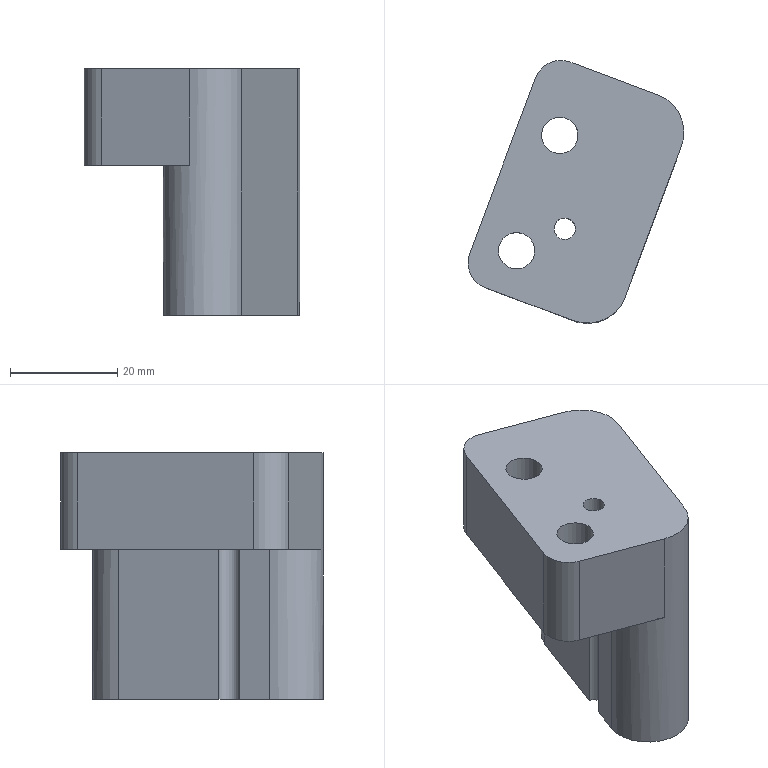Part | NX | features solid 2 | 1 solid | 24 faces | box 40.273 x 49.07 x 46 mm | volume 37890 mm3 | plane 11 | cylinder 11 | cone 2 | commonest cylinder face diameters 5.199 x2 6.8 x2 10 x2 11 x2 15 x2 4.001 x1
STEP:
#1=CARTESIAN_POINT('',(340.887,34.527,53.));
#2=VERTEX_POINT('',#1);
#3=CARTESIAN_POINT('',(336.736,38.135,53.));
#4=DIRECTION('',(0.000000102,-0.000000038,1.));
#5=DIRECTION('',(0.7547,-0.6561,-0.000000102));
#6=AXIS2_PLACEMENT_3D('',#3,#4,#5);
#7=CIRCLE('',#6,5.5);
#8=EDGE_CURVE('',#2,#2,#7,.T.);
#9=ORIENTED_EDGE('',*,*,#8,.T.);
#10=EDGE_LOOP('',(#9));
#11=FACE_BOUND('',#10,.T.);
#12=CARTESIAN_POINT('',(342.943,34.747,53.));
#13=VERTEX_POINT('',#12);
#14=CARTESIAN_POINT('',(345.044,40.367,53.));
#15=VERTEX_POINT('',#14);
#16=CARTESIAN_POINT('',(344.256,38.26,53.));
#17=DIRECTION('',(0.3502,0.9367,0.));
#18=VECTOR('',#17,1000.);
#19=LINE('',#16,#18);
#20=EDGE_CURVE('',#13,#15,#19,.T.);
#21=ORIENTED_EDGE('',*,*,#20,.F.);
#22=CARTESIAN_POINT('',(347.341,25.096,53.));
#23=VERTEX_POINT('',#22);
#24=CARTESIAN_POINT('',(349.968,32.121,53.));
#25=DIRECTION('',(0.,0.,-1.));
#26=DIRECTION('',(-1.,0.,0.));
#27=AXIS2_PLACEMENT_3D('',#24,#25,#26);
#28=CIRCLE('',#27,7.5);
#29=EDGE_CURVE('',#23,#13,#28,.T.);
#30=ORIENTED_EDGE('',*,*,#29,.F.);
#31=CARTESIAN_POINT('',(330.95,31.224,53.));
#32=VERTEX_POINT('',#31);
#33=CARTESIAN_POINT('',(328.608,32.1,53.));
#34=DIRECTION('',(0.9367,-0.3502,-0.000000109));
#35=VECTOR('',#34,1000.);
#36=LINE('',#33,#35);
#37=EDGE_CURVE('',#32,#23,#36,.T.);
#38=ORIENTED_EDGE('',*,*,#37,.F.);
#39=CARTESIAN_POINT('',(328.017,37.659,53.));
#40=VERTEX_POINT('',#39);
#41=CARTESIAN_POINT('',(332.701,35.908,53.));
#42=DIRECTION('',(0.000000102,-0.000000038,1.));
#43=DIRECTION('',(-1.,0.,0.000000102));
#44=AXIS2_PLACEMENT_3D('',#41,#42,#43);
#45=CIRCLE('',#44,5.);
#46=EDGE_CURVE('',#40,#32,#45,.T.);
#47=ORIENTED_EDGE('',*,*,#46,.F.);
#48=CARTESIAN_POINT('',(340.274,70.442,53.));
#49=VERTEX_POINT('',#48);
#50=CARTESIAN_POINT('',(362.919,131.008,53.));
#51=DIRECTION('',(-0.3502,-0.9367,0.));
#52=VECTOR('',#51,1000.);
#53=LINE('',#50,#52);
#54=EDGE_CURVE('',#49,#40,#53,.T.);
#55=ORIENTED_EDGE('',*,*,#54,.F.);
#56=CARTESIAN_POINT('',(346.709,73.375,53.));
#57=VERTEX_POINT('',#56);
#58=CARTESIAN_POINT('',(344.958,68.691,53.));
#59=DIRECTION('',(0.000000102,-0.000000038,1.));
#60=DIRECTION('',(-1.,0.,0.000000102));
#61=AXIS2_PLACEMENT_3D('',#58,#59,#60);
#62=CIRCLE('',#61,5.);
#63=EDGE_CURVE('',#57,#49,#62,.T.);
#64=ORIENTED_EDGE('',*,*,#63,.F.);
#65=CARTESIAN_POINT('',(363.101,67.246,53.));
#66=VERTEX_POINT('',#65);
#67=CARTESIAN_POINT('',(344.367,74.25,53.));
#68=DIRECTION('',(0.9367,-0.3502,-0.000000109));
#69=VECTOR('',#68,1000.);
#70=LINE('',#67,#69);
#71=EDGE_CURVE('',#57,#66,#70,.T.);
#72=ORIENTED_EDGE('',*,*,#71,.T.);
#73=CARTESIAN_POINT('',(353.449,62.847,53.));
#74=VERTEX_POINT('',#73);
#75=CARTESIAN_POINT('',(360.474,60.221,53.));
#76=DIRECTION('',(0.,0.,1.));
#77=DIRECTION('',(-1.,0.,0.));
#78=AXIS2_PLACEMENT_3D('',#75,#76,#77);
#79=CIRCLE('',#78,7.5);
#80=EDGE_CURVE('',#66,#74,#79,.T.);
#81=ORIENTED_EDGE('',*,*,#80,.T.);
#82=CARTESIAN_POINT('',(346.445,44.114,53.));
#83=VERTEX_POINT('',#82);
#84=CARTESIAN_POINT('',(344.256,38.26,53.));
#85=DIRECTION('',(0.3502,0.9367,0.));
#86=VECTOR('',#85,1000.);
#87=LINE('',#84,#86);
#88=EDGE_CURVE('',#83,#74,#87,.T.);
#89=ORIENTED_EDGE('',*,*,#88,.F.);
#90=CARTESIAN_POINT('',(345.744,42.241,53.));
#91=DIRECTION('',(-0.000000102,0.000000038,-1.));
#92=DIRECTION('',(-1.,0.,0.000000102));
#93=AXIS2_PLACEMENT_3D('',#90,#91,#92);
#94=CIRCLE('',#93,2.001);
#95=EDGE_CURVE('',#15,#83,#94,.T.);
#96=ORIENTED_EDGE('',*,*,#95,.F.);
#97=EDGE_LOOP('',(#21,#30,#38,#47,#55,#64,#72,#81,#89,#96));
#98=FACE_BOUND('',#97,.T.);
#99=CARTESIAN_POINT('',(350.291,59.679,53.));
#100=VERTEX_POINT('',#99);
#101=CARTESIAN_POINT('',(344.791,59.679,53.));
#102=DIRECTION('',(-0.000000102,0.000000038,-1.));
#103=DIRECTION('',(1.,0.,-0.000000102));
#104=AXIS2_PLACEMENT_3D('',#101,#102,#103);
#105=CIRCLE('',#104,5.5);
#106=EDGE_CURVE('',#100,#100,#105,.T.);
#107=ORIENTED_EDGE('',*,*,#106,.F.);
#108=EDGE_LOOP('',(#107));
#109=FACE_BOUND('',#108,.T.);
#110=CARTESIAN_POINT('',(365.26,130.133,53.));
#111=DIRECTION('',(-0.000000102,0.000000038,-1.));
#112=DIRECTION('',(1.,0.,-0.000000102));
#113=AXIS2_PLACEMENT_3D('',#110,#111,#112);
#114=PLANE('',#113);
#115=ADVANCED_FACE('',(#11,#98,#109),#114,.T.);
#116=CARTESIAN_POINT('',(340.136,38.135,71.));
#117=VERTEX_POINT('',#116);
#118=CARTESIAN_POINT('',(336.736,38.135,71.));
#119=DIRECTION('',(-0.000000102,0.000000038,-1.));
#120=DIRECTION('',(1.,0.,-0.000000102));
#121=AXIS2_PLACEMENT_3D('',#118,#119,#120);
#122=CIRCLE('',#121,3.4);
#123=EDGE_CURVE('',#117,#117,#122,.T.);
#124=ORIENTED_EDGE('',*,*,#123,.T.);
#125=EDGE_LOOP('',(#124));
#126=FACE_BOUND('',#125,.T.);
#127=CARTESIAN_POINT('',(330.95,31.224,71.));
#128=VERTEX_POINT('',#127);
#129=CARTESIAN_POINT('',(347.341,25.096,71.));
#130=VERTEX_POINT('',#129);
#131=CARTESIAN_POINT('',(328.608,32.1,71.));
#132=DIRECTION('',(0.9367,-0.3502,-0.000000109));
#133=VECTOR('',#132,1000.);
#134=LINE('',#131,#133);
#135=EDGE_CURVE('',#128,#130,#134,.T.);
#136=ORIENTED_EDGE('',*,*,#135,.T.);
#137=CARTESIAN_POINT('',(356.993,29.494,71.));
#138=VERTEX_POINT('',#137);
#139=CARTESIAN_POINT('',(349.968,32.121,71.));
#140=DIRECTION('',(0.,0.,1.));
#141=DIRECTION('',(1.,0.,0.));
#142=AXIS2_PLACEMENT_3D('',#139,#140,#141);
#143=CIRCLE('',#142,7.5);
#144=EDGE_CURVE('',#130,#138,#143,.T.);
#145=ORIENTED_EDGE('',*,*,#144,.T.);
#146=CARTESIAN_POINT('',(367.499,57.594,71.));
#147=VERTEX_POINT('',#146);
#148=CARTESIAN_POINT('',(358.306,33.007,71.));
#149=DIRECTION('',(0.3502,0.9367,0.));
#150=VECTOR('',#149,1000.);
#151=LINE('',#148,#150);
#152=EDGE_CURVE('',#138,#147,#151,.T.);
#153=ORIENTED_EDGE('',*,*,#152,.T.);
#154=CARTESIAN_POINT('',(363.101,67.246,71.));
#155=VERTEX_POINT('',#154);
#156=CARTESIAN_POINT('',(360.474,60.221,71.));
#157=DIRECTION('',(0.,0.,1.));
#158=DIRECTION('',(1.,0.,0.));
#159=AXIS2_PLACEMENT_3D('',#156,#157,#158);
#160=CIRCLE('',#159,7.5);
#161=EDGE_CURVE('',#147,#155,#160,.T.);
#162=ORIENTED_EDGE('',*,*,#161,.T.);
#163=CARTESIAN_POINT('',(346.709,73.375,71.));
#164=VERTEX_POINT('',#163);
#165=CARTESIAN_POINT('',(344.367,74.25,71.));
#166=DIRECTION('',(0.9367,-0.3502,-0.000000109));
#167=VECTOR('',#166,1000.);
#168=LINE('',#165,#167);
#169=EDGE_CURVE('',#164,#155,#168,.T.);
#170=ORIENTED_EDGE('',*,*,#169,.F.);
#171=CARTESIAN_POINT('',(340.274,70.442,71.));
#172=VERTEX_POINT('',#171);
#173=CARTESIAN_POINT('',(344.958,68.691,71.));
#174=DIRECTION('',(-0.000000102,0.000000038,-1.));
#175=DIRECTION('',(1.,0.,-0.000000102));
#176=AXIS2_PLACEMENT_3D('',#173,#174,#175);
#177=CIRCLE('',#176,5.);
#178=EDGE_CURVE('',#172,#164,#177,.T.);
#179=ORIENTED_EDGE('',*,*,#178,.F.);
#180=CARTESIAN_POINT('',(328.017,37.659,71.));
#181=VERTEX_POINT('',#180);
#182=CARTESIAN_POINT('',(362.919,131.008,71.));
#183=DIRECTION('',(0.3502,0.9367,0.));
#184=VECTOR('',#183,1000.);
#185=LINE('',#182,#184);
#186=EDGE_CURVE('',#181,#172,#185,.T.);
#187=ORIENTED_EDGE('',*,*,#186,.F.);
#188=CARTESIAN_POINT('',(332.701,35.908,71.));
#189=DIRECTION('',(-0.000000102,0.000000038,-1.));
#190=DIRECTION('',(1.,0.,-0.000000102));
#191=AXIS2_PLACEMENT_3D('',#188,#189,#190);
#192=CIRCLE('',#191,5.);
#193=EDGE_CURVE('',#128,#181,#192,.T.);
#194=ORIENTED_EDGE('',*,*,#193,.F.);
#195=EDGE_LOOP('',(#136,#145,#153,#162,#170,#179,#187,#194));
#196=FACE_BOUND('',#195,.T.);
#197=CARTESIAN_POINT('',(347.745,42.241,71.));
#198=VERTEX_POINT('',#197);
#199=CARTESIAN_POINT('',(345.744,42.241,71.));
#200=DIRECTION('',(-0.000000102,0.000000038,-1.));
#201=DIRECTION('',(1.,0.,-0.000000102));
#202=AXIS2_PLACEMENT_3D('',#199,#200,#201);
#203=CIRCLE('',#202,2.001);
#204=EDGE_CURVE('',#198,#198,#203,.T.);
#205=ORIENTED_EDGE('',*,*,#204,.T.);
#206=EDGE_LOOP('',(#205));
#207=FACE_BOUND('',#206,.T.);
#208=CARTESIAN_POINT('',(348.191,59.679,71.));
#209=VERTEX_POINT('',#208);
#210=CARTESIAN_POINT('',(344.791,59.679,71.));
#211=DIRECTION('',(0.000000102,-0.000000038,1.));
#212=DIRECTION('',(1.,0.,-0.000000102));
#213=AXIS2_PLACEMENT_3D('',#210,#211,#212);
#214=CIRCLE('',#213,3.4);
#215=EDGE_CURVE('',#209,#209,#214,.T.);
#216=ORIENTED_EDGE('',*,*,#215,.F.);
#217=EDGE_LOOP('',(#216));
#218=FACE_BOUND('',#217,.T.);
#219=CARTESIAN_POINT('',(365.26,130.133,71.));
#220=DIRECTION('',(0.000000102,-0.000000038,1.));
#221=DIRECTION('',(-1.,0.,0.000000102));
#222=AXIS2_PLACEMENT_3D('',#219,#220,#221);
#223=PLANE('',#222);
#224=ADVANCED_FACE('',(#126,#196,#207,#218),#223,.T.);
#225=CARTESIAN_POINT('',(346.445,44.114,25.));
#226=VERTEX_POINT('',#225);
#227=CARTESIAN_POINT('',(346.445,44.114,15.));
#228=DIRECTION('',(0.000000103,-0.000000037,1.));
#229=VECTOR('',#228,1000.);
#230=LINE('',#227,#229);
#231=EDGE_CURVE('',#226,#83,#230,.T.);
#232=ORIENTED_EDGE('',*,*,#231,.T.);
#233=ORIENTED_EDGE('',*,*,#88,.T.);
#234=CARTESIAN_POINT('',(353.449,62.847,25.));
#235=VERTEX_POINT('',#234);
#236=CARTESIAN_POINT('',(353.449,62.847,65.));
#237=DIRECTION('',(-0.000000103,0.000000037,-1.));
#238=VECTOR('',#237,1000.);
#239=LINE('',#236,#238);
#240=EDGE_CURVE('',#74,#235,#239,.T.);
#241=ORIENTED_EDGE('',*,*,#240,.T.);
#242=CARTESIAN_POINT('',(344.256,38.26,25.));
#243=DIRECTION('',(0.3502,0.9367,-0.000000001));
#244=VECTOR('',#243,1000.);
#245=LINE('',#242,#244);
#246=EDGE_CURVE('',#226,#235,#245,.T.);
#247=ORIENTED_EDGE('',*,*,#246,.F.);
#248=EDGE_LOOP('',(#232,#233,#241,#247));
#249=FACE_BOUND('',#248,.T.);
#250=CARTESIAN_POINT('',(344.256,38.26,65.));
#251=DIRECTION('',(0.9367,-0.3502,-0.000000109));
#252=DIRECTION('',(0.3502,0.9367,0.));
#253=AXIS2_PLACEMENT_3D('',#250,#251,#252);
#254=PLANE('',#253);
#255=ADVANCED_FACE('',(#249),#254,.F.);
#256=CARTESIAN_POINT('',(345.044,40.367,25.));
#257=VERTEX_POINT('',#256);
#258=CARTESIAN_POINT('',(345.044,40.367,15.));
#259=DIRECTION('',(-0.000000103,0.000000037,-1.));
#260=VECTOR('',#259,1000.);
#261=LINE('',#258,#260);
#262=EDGE_CURVE('',#15,#257,#261,.T.);
#263=ORIENTED_EDGE('',*,*,#262,.T.);
#264=CARTESIAN_POINT('',(342.943,34.747,25.));
#265=VERTEX_POINT('',#264);
#266=CARTESIAN_POINT('',(344.256,38.26,25.));
#267=DIRECTION('',(0.3502,0.9367,-0.000000001));
#268=VECTOR('',#267,1000.);
#269=LINE('',#266,#268);
#270=EDGE_CURVE('',#265,#257,#269,.T.);
#271=ORIENTED_EDGE('',*,*,#270,.F.);
#272=CARTESIAN_POINT('',(342.943,34.747,65.));
#273=DIRECTION('',(-0.000000103,0.000000037,-1.));
#274=VECTOR('',#273,1000.);
#275=LINE('',#272,#274);
#276=EDGE_CURVE('',#13,#265,#275,.T.);
#277=ORIENTED_EDGE('',*,*,#276,.F.);
#278=ORIENTED_EDGE('',*,*,#20,.T.);
#279=EDGE_LOOP('',(#263,#271,#277,#278));
#280=FACE_BOUND('',#279,.T.);
#281=CARTESIAN_POINT('',(344.256,38.26,65.));
#282=DIRECTION('',(0.9367,-0.3502,-0.000000109));
#283=DIRECTION('',(0.3502,0.9367,0.));
#284=AXIS2_PLACEMENT_3D('',#281,#282,#283);
#285=PLANE('',#284);
#286=ADVANCED_FACE('',(#280),#285,.F.);
#287=CARTESIAN_POINT('',(352.568,32.121,25.));
#288=VERTEX_POINT('',#287);
#289=CARTESIAN_POINT('',(349.968,32.121,25.));
#290=DIRECTION('',(0.000000103,-0.000000037,1.));
#291=DIRECTION('',(1.,0.,-0.000000103));
#292=AXIS2_PLACEMENT_3D('',#289,#290,#291);
#293=CIRCLE('',#292,2.599);
#294=EDGE_CURVE('',#288,#288,#293,.T.);
#295=ORIENTED_EDGE('',*,*,#294,.T.);
#296=EDGE_LOOP('',(#295));
#297=FACE_BOUND('',#296,.T.);
#298=CARTESIAN_POINT('',(363.074,60.221,25.));
#299=VERTEX_POINT('',#298);
#300=CARTESIAN_POINT('',(360.474,60.221,25.));
#301=DIRECTION('',(0.000000103,-0.000000037,1.));
#302=DIRECTION('',(1.,0.,-0.000000103));
#303=AXIS2_PLACEMENT_3D('',#300,#301,#302);
#304=CIRCLE('',#303,2.599);
#305=EDGE_CURVE('',#299,#299,#304,.T.);
#306=ORIENTED_EDGE('',*,*,#305,.T.);
#307=EDGE_LOOP('',(#306));
#308=FACE_BOUND('',#307,.T.);
#309=CARTESIAN_POINT('',(345.744,42.241,25.));
#310=DIRECTION('',(0.000000103,-0.000000037,1.));
#311=DIRECTION('',(1.,0.,-0.000000103));
#312=AXIS2_PLACEMENT_3D('',#309,#310,#311);
#313=CIRCLE('',#312,2.001);
#314=EDGE_CURVE('',#257,#226,#313,.T.);
#315=ORIENTED_EDGE('',*,*,#314,.T.);
#316=ORIENTED_EDGE('',*,*,#246,.T.);
#317=CARTESIAN_POINT('',(367.499,57.594,25.));
#318=VERTEX_POINT('',#317);
#319=CARTESIAN_POINT('',(360.474,60.221,25.));
#320=DIRECTION('',(0.000000103,-0.000000037,1.));
#321=DIRECTION('',(1.,0.,-0.000000103));
#322=AXIS2_PLACEMENT_3D('',#319,#320,#321);
#323=CIRCLE('',#322,7.5);
#324=EDGE_CURVE('',#318,#235,#323,.T.);
#325=ORIENTED_EDGE('',*,*,#324,.F.);
#326=CARTESIAN_POINT('',(356.993,29.494,25.));
#327=VERTEX_POINT('',#326);
#328=CARTESIAN_POINT('',(358.306,33.007,25.));
#329=DIRECTION('',(0.3502,0.9367,-0.000000001));
#330=VECTOR('',#329,1000.);
#331=LINE('',#328,#330);
#332=EDGE_CURVE('',#327,#318,#331,.T.);
#333=ORIENTED_EDGE('',*,*,#332,.F.);
#334=CARTESIAN_POINT('',(349.968,32.121,25.));
#335=DIRECTION('',(0.000000103,-0.000000037,1.));
#336=DIRECTION('',(1.,0.,-0.000000103));
#337=AXIS2_PLACEMENT_3D('',#334,#335,#336);
#338=CIRCLE('',#337,7.5);
#339=EDGE_CURVE('',#265,#327,#338,.T.);
#340=ORIENTED_EDGE('',*,*,#339,.F.);
#341=ORIENTED_EDGE('',*,*,#270,.T.);
#342=EDGE_LOOP('',(#315,#316,#325,#333,#340,#341));
#343=FACE_BOUND('',#342,.T.);
#344=CARTESIAN_POINT('',(351.281,35.633,25.));
#345=DIRECTION('',(0.000000103,-0.000000037,1.));
#346=DIRECTION('',(-0.04361,-0.999,-0.000000033));
#347=AXIS2_PLACEMENT_3D('',#344,#345,#346);
#348=PLANE('',#347);
#349=ADVANCED_FACE('',(#297,#308,#343),#348,.F.);
#350=ORIENTED_EDGE('',*,*,#29,.T.);
#351=ORIENTED_EDGE('',*,*,#276,.T.);
#352=ORIENTED_EDGE('',*,*,#339,.T.);
#353=CARTESIAN_POINT('',(356.993,29.494,65.));
#354=DIRECTION('',(-0.000000103,0.000000037,-1.));
#355=VECTOR('',#354,1000.);
#356=LINE('',#353,#355);
#357=EDGE_CURVE('',#138,#327,#356,.T.);
#358=ORIENTED_EDGE('',*,*,#357,.F.);
#359=ORIENTED_EDGE('',*,*,#144,.F.);
#360=CARTESIAN_POINT('',(347.341,25.096,65.));
#361=DIRECTION('',(0.000000103,-0.000000037,1.));
#362=VECTOR('',#361,1000.);
#363=LINE('',#360,#362);
#364=EDGE_CURVE('',#23,#130,#363,.T.);
#365=ORIENTED_EDGE('',*,*,#364,.F.);
#366=EDGE_LOOP('',(#350,#351,#352,#358,#359,#365));
#367=FACE_BOUND('',#366,.T.);
#368=CARTESIAN_POINT('',(349.968,32.121,65.));
#369=DIRECTION('',(-0.000000103,0.000000037,-1.));
#370=DIRECTION('',(1.,0.,-0.000000103));
#371=AXIS2_PLACEMENT_3D('',#368,#369,#370);
#372=CYLINDRICAL_SURFACE('',#371,7.5);
#373=ADVANCED_FACE('',(#367),#372,.T.);
#374=CARTESIAN_POINT('',(367.499,57.594,65.));
#375=DIRECTION('',(-0.000000103,0.000000037,-1.));
#376=VECTOR('',#375,1000.);
#377=LINE('',#374,#376);
#378=EDGE_CURVE('',#147,#318,#377,.T.);
#379=ORIENTED_EDGE('',*,*,#378,.T.);
#380=ORIENTED_EDGE('',*,*,#324,.T.);
#381=ORIENTED_EDGE('',*,*,#240,.F.);
#382=ORIENTED_EDGE('',*,*,#80,.F.);
#383=CARTESIAN_POINT('',(363.101,67.246,65.));
#384=DIRECTION('',(-0.000000103,0.000000037,-1.));
#385=VECTOR('',#384,1000.);
#386=LINE('',#383,#385);
#387=EDGE_CURVE('',#155,#66,#386,.T.);
#388=ORIENTED_EDGE('',*,*,#387,.F.);
#389=ORIENTED_EDGE('',*,*,#161,.F.);
#390=EDGE_LOOP('',(#379,#380,#381,#382,#388,#389));
#391=FACE_BOUND('',#390,.T.);
#392=CARTESIAN_POINT('',(360.474,60.221,65.));
#393=DIRECTION('',(-0.000000103,0.000000037,-1.));
#394=DIRECTION('',(1.,0.,-0.000000103));
#395=AXIS2_PLACEMENT_3D('',#392,#393,#394);
#396=CYLINDRICAL_SURFACE('',#395,7.5);
#397=ADVANCED_FACE('',(#391),#396,.T.);
#398=ORIENTED_EDGE('',*,*,#357,.T.);
#399=ORIENTED_EDGE('',*,*,#332,.T.);
#400=ORIENTED_EDGE('',*,*,#378,.F.);
#401=ORIENTED_EDGE('',*,*,#152,.F.);
#402=EDGE_LOOP('',(#398,#399,#400,#401));
#403=FACE_BOUND('',#402,.T.);
#404=CARTESIAN_POINT('',(358.306,33.007,65.));
#405=DIRECTION('',(0.9367,-0.3502,-0.000000109));
#406=DIRECTION('',(0.3502,0.9367,0.));
#407=AXIS2_PLACEMENT_3D('',#404,#405,#406);
#408=PLANE('',#407);
#409=ADVANCED_FACE('',(#403),#408,.T.);
#410=ORIENTED_EDGE('',*,*,#169,.T.);
#411=ORIENTED_EDGE('',*,*,#387,.T.);
#412=ORIENTED_EDGE('',*,*,#71,.F.);
#413=CARTESIAN_POINT('',(346.709,73.375,65.));
#414=DIRECTION('',(-0.000000103,0.000000037,-1.));
#415=VECTOR('',#414,1000.);
#416=LINE('',#413,#415);
#417=EDGE_CURVE('',#164,#57,#416,.T.);
#418=ORIENTED_EDGE('',*,*,#417,.F.);
#419=EDGE_LOOP('',(#410,#411,#412,#418));
#420=FACE_BOUND('',#419,.T.);
#421=CARTESIAN_POINT('',(344.367,74.25,65.));
#422=DIRECTION('',(0.3502,0.9367,-0.000000001));
#423=DIRECTION('',(-0.9367,0.3502,0.));
#424=AXIS2_PLACEMENT_3D('',#421,#422,#423);
#425=PLANE('',#424);
#426=ADVANCED_FACE('',(#420),#425,.T.);
#427=ORIENTED_EDGE('',*,*,#37,.T.);
#428=ORIENTED_EDGE('',*,*,#364,.T.);
#429=ORIENTED_EDGE('',*,*,#135,.F.);
#430=CARTESIAN_POINT('',(330.95,31.224,65.));
#431=DIRECTION('',(0.000000103,-0.000000037,1.));
#432=VECTOR('',#431,1000.);
#433=LINE('',#430,#432);
#434=EDGE_CURVE('',#32,#128,#433,.T.);
#435=ORIENTED_EDGE('',*,*,#434,.F.);
#436=EDGE_LOOP('',(#427,#428,#429,#435));
#437=FACE_BOUND('',#436,.T.);
#438=CARTESIAN_POINT('',(328.608,32.1,65.));
#439=DIRECTION('',(-0.3502,-0.9367,0.000000001));
#440=DIRECTION('',(0.9367,-0.3502,0.));
#441=AXIS2_PLACEMENT_3D('',#438,#439,#440);
#442=PLANE('',#441);
#443=ADVANCED_FACE('',(#437),#442,.T.);
#444=ORIENTED_EDGE('',*,*,#186,.T.);
#445=CARTESIAN_POINT('',(340.274,70.442,53.));
#446=DIRECTION('',(0.000000103,-0.000000037,1.));
#447=VECTOR('',#446,1000.);
#448=LINE('',#445,#447);
#449=EDGE_CURVE('',#49,#172,#448,.T.);
#450=ORIENTED_EDGE('',*,*,#449,.F.);
#451=ORIENTED_EDGE('',*,*,#54,.T.);
#452=CARTESIAN_POINT('',(328.017,37.659,53.));
#453=DIRECTION('',(-0.000000103,0.000000037,-1.));
#454=VECTOR('',#453,1000.);
#455=LINE('',#452,#454);
#456=EDGE_CURVE('',#181,#40,#455,.T.);
#457=ORIENTED_EDGE('',*,*,#456,.F.);
#458=EDGE_LOOP('',(#444,#450,#451,#457));
#459=FACE_BOUND('',#458,.T.);
#460=CARTESIAN_POINT('',(328.893,40.,53.));
#461=DIRECTION('',(-0.9367,0.3502,0.000000109));
#462=DIRECTION('',(-0.3502,-0.9367,0.));
#463=AXIS2_PLACEMENT_3D('',#460,#461,#462);
#464=PLANE('',#463);
#465=ADVANCED_FACE('',(#459),#464,.T.);
#466=ORIENTED_EDGE('',*,*,#46,.T.);
#467=ORIENTED_EDGE('',*,*,#434,.T.);
#468=ORIENTED_EDGE('',*,*,#193,.T.);
#469=ORIENTED_EDGE('',*,*,#456,.T.);
#470=EDGE_LOOP('',(#466,#467,#468,#469));
#471=FACE_BOUND('',#470,.T.);
#472=CARTESIAN_POINT('',(332.701,35.908,65.));
#473=DIRECTION('',(0.000000103,-0.000000037,1.));
#474=DIRECTION('',(-1.,0.,0.000000103));
#475=AXIS2_PLACEMENT_3D('',#472,#473,#474);
#476=CYLINDRICAL_SURFACE('',#475,5.);
#477=ADVANCED_FACE('',(#471),#476,.T.);
#478=ORIENTED_EDGE('',*,*,#178,.T.);
#479=ORIENTED_EDGE('',*,*,#417,.T.);
#480=ORIENTED_EDGE('',*,*,#63,.T.);
#481=ORIENTED_EDGE('',*,*,#449,.T.);
#482=EDGE_LOOP('',(#478,#479,#480,#481));
#483=FACE_BOUND('',#482,.T.);
#484=CARTESIAN_POINT('',(344.958,68.691,65.));
#485=DIRECTION('',(-0.000000103,0.000000037,-1.));
#486=DIRECTION('',(1.,0.,-0.000000103));
#487=AXIS2_PLACEMENT_3D('',#484,#485,#486);
#488=CYLINDRICAL_SURFACE('',#487,5.);
#489=ADVANCED_FACE('',(#483),#488,.T.);
#490=ORIENTED_EDGE('',*,*,#204,.F.);
#491=EDGE_LOOP('',(#490));
#492=FACE_BOUND('',#491,.T.);
#493=ORIENTED_EDGE('',*,*,#314,.F.);
#494=ORIENTED_EDGE('',*,*,#262,.F.);
#495=ORIENTED_EDGE('',*,*,#95,.T.);
#496=ORIENTED_EDGE('',*,*,#231,.F.);
#497=EDGE_LOOP('',(#493,#494,#495,#496));
#498=FACE_BOUND('',#497,.T.);
#499=CARTESIAN_POINT('',(345.744,42.241,15.));
#500=DIRECTION('',(-0.000000103,0.000000037,-1.));
#501=DIRECTION('',(1.,0.,-0.000000103));
#502=AXIS2_PLACEMENT_3D('',#499,#500,#501);
#503=CYLINDRICAL_SURFACE('',#502,2.001);
#504=ADVANCED_FACE('',(#492,#498),#503,.F.);
#505=CARTESIAN_POINT('',(348.191,59.679,62.));
#506=VERTEX_POINT('',#505);
#507=CARTESIAN_POINT('',(344.791,59.679,62.));
#508=DIRECTION('',(-0.000000102,0.000000038,-1.));
#509=DIRECTION('',(1.,0.,-0.000000102));
#510=AXIS2_PLACEMENT_3D('',#507,#508,#509);
#511=CIRCLE('',#510,3.4);
#512=EDGE_CURVE('',#506,#506,#511,.T.);
#513=ORIENTED_EDGE('',*,*,#512,.T.);
#514=EDGE_LOOP('',(#513));
#515=FACE_BOUND('',#514,.T.);
#516=ORIENTED_EDGE('',*,*,#215,.T.);
#517=EDGE_LOOP('',(#516));
#518=FACE_BOUND('',#517,.T.);
#519=CARTESIAN_POINT('',(344.791,59.679,53.));
#520=DIRECTION('',(0.000000102,-0.000000038,1.));
#521=DIRECTION('',(-1.,0.,0.000000102));
#522=AXIS2_PLACEMENT_3D('',#519,#520,#521);
#523=CYLINDRICAL_SURFACE('',#522,3.4);
#524=ADVANCED_FACE('',(#515,#518),#523,.F.);
#525=ORIENTED_EDGE('',*,*,#512,.F.);
#526=EDGE_LOOP('',(#525));
#527=FACE_BOUND('',#526,.T.);
#528=CARTESIAN_POINT('',(350.291,59.679,62.));
#529=VERTEX_POINT('',#528);
#530=CARTESIAN_POINT('',(344.791,59.679,62.));
#531=DIRECTION('',(-0.000000102,0.000000038,-1.));
#532=DIRECTION('',(1.,0.,-0.000000102));
#533=AXIS2_PLACEMENT_3D('',#530,#531,#532);
#534=CIRCLE('',#533,5.5);
#535=EDGE_CURVE('',#529,#529,#534,.T.);
#536=ORIENTED_EDGE('',*,*,#535,.T.);
#537=EDGE_LOOP('',(#536));
#538=FACE_BOUND('',#537,.T.);
#539=CARTESIAN_POINT('',(344.791,59.679,62.));
#540=DIRECTION('',(0.000000102,-0.000000038,1.));
#541=DIRECTION('',(-1.,0.,0.000000102));
#542=AXIS2_PLACEMENT_3D('',#539,#540,#541);
#543=PLANE('',#542);
#544=ADVANCED_FACE('',(#527,#538),#543,.F.);
#545=ORIENTED_EDGE('',*,*,#535,.F.);
#546=EDGE_LOOP('',(#545));
#547=FACE_BOUND('',#546,.T.);
#548=ORIENTED_EDGE('',*,*,#106,.T.);
#549=EDGE_LOOP('',(#548));
#550=FACE_BOUND('',#549,.T.);
#551=CARTESIAN_POINT('',(344.791,59.679,53.));
#552=DIRECTION('',(0.000000102,-0.000000038,1.));
#553=DIRECTION('',(-1.,0.,0.000000102));
#554=AXIS2_PLACEMENT_3D('',#551,#552,#553);
#555=CYLINDRICAL_SURFACE('',#554,5.5);
#556=ADVANCED_FACE('',(#547,#550),#555,.F.);
#557=CARTESIAN_POINT('',(340.136,38.135,62.));
#558=VERTEX_POINT('',#557);
#559=CARTESIAN_POINT('',(336.736,38.135,62.));
#560=DIRECTION('',(0.000000102,-0.000000038,1.));
#561=DIRECTION('',(1.,0.,-0.000000102));
#562=AXIS2_PLACEMENT_3D('',#559,#560,#561);
#563=CIRCLE('',#562,3.4);
#564=EDGE_CURVE('',#558,#558,#563,.T.);
#565=ORIENTED_EDGE('',*,*,#564,.F.);
#566=EDGE_LOOP('',(#565));
#567=FACE_BOUND('',#566,.T.);
#568=ORIENTED_EDGE('',*,*,#123,.F.);
#569=EDGE_LOOP('',(#568));
#570=FACE_BOUND('',#569,.T.);
#571=CARTESIAN_POINT('',(336.736,38.135,53.));
#572=DIRECTION('',(0.000000102,-0.000000038,1.));
#573=DIRECTION('',(-0.7547,0.6561,0.000000102));
#574=AXIS2_PLACEMENT_3D('',#571,#572,#573);
#575=CYLINDRICAL_SURFACE('',#574,3.4);
#576=ADVANCED_FACE('',(#567,#570),#575,.F.);
#577=ORIENTED_EDGE('',*,*,#564,.T.);
#578=EDGE_LOOP('',(#577));
#579=FACE_BOUND('',#578,.T.);
#580=CARTESIAN_POINT('',(340.887,34.527,62.));
#581=VERTEX_POINT('',#580);
#582=CARTESIAN_POINT('',(336.736,38.135,62.));
#583=DIRECTION('',(0.000000102,-0.000000038,1.));
#584=DIRECTION('',(0.7547,-0.6561,-0.000000102));
#585=AXIS2_PLACEMENT_3D('',#582,#583,#584);
#586=CIRCLE('',#585,5.5);
#587=EDGE_CURVE('',#581,#581,#586,.T.);
#588=ORIENTED_EDGE('',*,*,#587,.F.);
#589=EDGE_LOOP('',(#588));
#590=FACE_BOUND('',#589,.T.);
#591=CARTESIAN_POINT('',(336.736,38.135,62.));
#592=DIRECTION('',(0.000000102,-0.000000038,1.));
#593=DIRECTION('',(-0.7547,0.6561,0.000000102));
#594=AXIS2_PLACEMENT_3D('',#591,#592,#593);
#595=PLANE('',#594);
#596=ADVANCED_FACE('',(#579,#590),#595,.F.);
#597=ORIENTED_EDGE('',*,*,#587,.T.);
#598=EDGE_LOOP('',(#597));
#599=FACE_BOUND('',#598,.T.);
#600=ORIENTED_EDGE('',*,*,#8,.F.);
#601=EDGE_LOOP('',(#600));
#602=FACE_BOUND('',#601,.T.);
#603=CARTESIAN_POINT('',(336.736,38.135,53.));
#604=DIRECTION('',(0.000000102,-0.000000038,1.));
#605=DIRECTION('',(-0.7547,0.6561,0.000000102));
#606=AXIS2_PLACEMENT_3D('',#603,#604,#605);
#607=CYLINDRICAL_SURFACE('',#606,5.5);
#608=ADVANCED_FACE('',(#599,#602),#607,.F.);
#609=CARTESIAN_POINT('',(363.074,60.221,37.401));
#610=VERTEX_POINT('',#609);
#611=CARTESIAN_POINT('',(360.474,60.221,37.401));
#612=DIRECTION('',(0.000000103,-0.000000037,1.));
#613=DIRECTION('',(1.,0.,-0.000000103));
#614=AXIS2_PLACEMENT_3D('',#611,#612,#613);
#615=CIRCLE('',#614,2.599);
#616=EDGE_CURVE('',#610,#610,#615,.T.);
#617=ORIENTED_EDGE('',*,*,#616,.T.);
#618=EDGE_LOOP('',(#617));
#619=FACE_BOUND('',#618,.T.);
#620=ORIENTED_EDGE('',*,*,#305,.F.);
#621=EDGE_LOOP('',(#620));
#622=FACE_BOUND('',#621,.T.);
#623=CARTESIAN_POINT('',(360.474,60.221,25.));
#624=DIRECTION('',(0.000000103,-0.000000037,1.));
#625=DIRECTION('',(-1.,0.,0.000000103));
#626=AXIS2_PLACEMENT_3D('',#623,#624,#625);
#627=CYLINDRICAL_SURFACE('',#626,2.599);
#628=ADVANCED_FACE('',(#619,#622),#627,.F.);
#629=CARTESIAN_POINT('',(360.474,60.221,40.));
#630=VERTEX_POINT('',#629);
#631=VERTEX_LOOP('',#630);
#632=FACE_BOUND('',#631,.T.);
#633=ORIENTED_EDGE('',*,*,#616,.F.);
#634=EDGE_LOOP('',(#633));
#635=FACE_BOUND('',#634,.T.);
#636=CARTESIAN_POINT('',(360.474,60.221,37.401));
#637=DIRECTION('',(-0.000000103,0.000000037,-1.));
#638=DIRECTION('',(1.,0.,-0.000000103));
#639=AXIS2_PLACEMENT_3D('',#636,#637,#638);
#640=CONICAL_SURFACE('',#639,2.599,0.7854);
#641=ADVANCED_FACE('',(#632,#635),#640,.F.);
#642=CARTESIAN_POINT('',(352.568,32.121,37.401));
#643=VERTEX_POINT('',#642);
#644=CARTESIAN_POINT('',(349.968,32.121,37.401));
#645=DIRECTION('',(0.000000103,-0.000000037,1.));
#646=DIRECTION('',(1.,0.,-0.000000103));
#647=AXIS2_PLACEMENT_3D('',#644,#645,#646);
#648=CIRCLE('',#647,2.599);
#649=EDGE_CURVE('',#643,#643,#648,.T.);
#650=ORIENTED_EDGE('',*,*,#649,.T.);
#651=EDGE_LOOP('',(#650));
#652=FACE_BOUND('',#651,.T.);
#653=ORIENTED_EDGE('',*,*,#294,.F.);
#654=EDGE_LOOP('',(#653));
#655=FACE_BOUND('',#654,.T.);
#656=CARTESIAN_POINT('',(349.968,32.121,25.));
#657=DIRECTION('',(0.000000103,-0.000000037,1.));
#658=DIRECTION('',(-1.,0.,0.000000103));
#659=AXIS2_PLACEMENT_3D('',#656,#657,#658);
#660=CYLINDRICAL_SURFACE('',#659,2.599);
#661=ADVANCED_FACE('',(#652,#655),#660,.F.);
#662=CARTESIAN_POINT('',(349.968,32.121,40.));
#663=VERTEX_POINT('',#662);
#664=VERTEX_LOOP('',#663);
#665=FACE_BOUND('',#664,.T.);
#666=ORIENTED_EDGE('',*,*,#649,.F.);
#667=EDGE_LOOP('',(#666));
#668=FACE_BOUND('',#667,.T.);
#669=CARTESIAN_POINT('',(349.968,32.121,37.401));
#670=DIRECTION('',(-0.000000103,0.000000037,-1.));
#671=DIRECTION('',(1.,0.,-0.000000103));
#672=AXIS2_PLACEMENT_3D('',#669,#670,#671);
#673=CONICAL_SURFACE('',#672,2.599,0.7854);
#674=ADVANCED_FACE('',(#665,#668),#673,.F.);
#675=CLOSED_SHELL('',(#115,#224,#255,#286,#349,#373,#397,#409,#426,#443,#465,#477,#489,#504,#524,#544,#556,#576,#596,#608,#628,#641,#661,#674));
#676=MANIFOLD_SOLID_BREP('',#675);
#677=(LENGTH_UNIT()NAMED_UNIT(*)SI_UNIT(.MILLI.,.METRE.));
#678=UNCERTAINTY_MEASURE_WITH_UNIT(LENGTH_MEASURE(0.00001),#677,'','');
#679=(NAMED_UNIT(*)PLANE_ANGLE_UNIT()SI_UNIT($,.RADIAN.));
#680=(NAMED_UNIT(*)SI_UNIT($,.STERADIAN.)SOLID_ANGLE_UNIT());
#681=(GEOMETRIC_REPRESENTATION_CONTEXT(3)GLOBAL_UNCERTAINTY_ASSIGNED_CONTEXT((#678))GLOBAL_UNIT_ASSIGNED_CONTEXT((#677,#679,#680))REPRESENTATION_CONTEXT('',''));
#682=ADVANCED_BREP_SHAPE_REPRESENTATION('',(#676),#681);